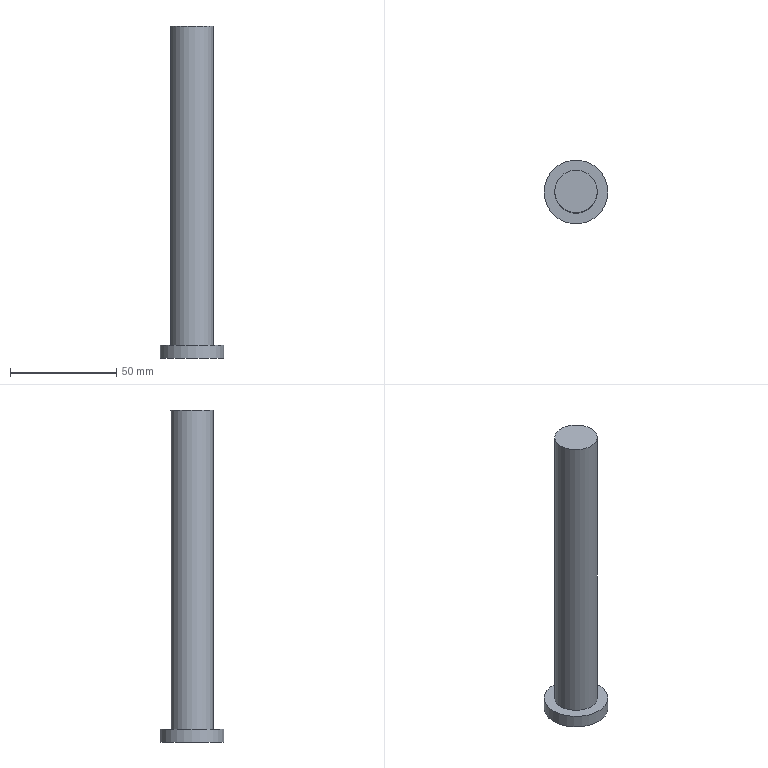Part | NX | features 侧推千斤顶活塞销 2 | 1 solid | 5 faces | box 30 x 30 x 156 mm | volume 51365 mm3 | plane 3 | cylinder 2 | commonest cylinder face diameters 20 x1 30 x1
STEP:
#1=CARTESIAN_POINT('',(10.,0.,150.));
#2=VERTEX_POINT('',#1);
#3=CARTESIAN_POINT('',(0.,0.,150.));
#4=DIRECTION('',(0.,0.,1.));
#5=DIRECTION('',(1.,0.,0.));
#6=AXIS2_PLACEMENT_3D('',#3,#4,#5);
#7=CIRCLE('',#6,10.);
#8=EDGE_CURVE('',#2,#2,#7,.T.);
#9=ORIENTED_EDGE('',*,*,#8,.F.);
#10=EDGE_LOOP('',(#9));
#11=FACE_BOUND('',#10,.T.);
#12=CARTESIAN_POINT('',(-10.,0.,0.));
#13=VERTEX_POINT('',#12);
#14=CARTESIAN_POINT('',(0.,0.,0.));
#15=DIRECTION('',(0.,0.,-1.));
#16=DIRECTION('',(-1.,0.,0.));
#17=AXIS2_PLACEMENT_3D('',#14,#15,#16);
#18=CIRCLE('',#17,10.);
#19=EDGE_CURVE('',#13,#13,#18,.T.);
#20=ORIENTED_EDGE('',*,*,#19,.F.);
#21=EDGE_LOOP('',(#20));
#22=FACE_BOUND('',#21,.T.);
#23=CARTESIAN_POINT('',(0.,0.,150.));
#24=DIRECTION('',(0.,0.,-1.));
#25=DIRECTION('',(-1.,0.,0.));
#26=AXIS2_PLACEMENT_3D('',#23,#24,#25);
#27=CYLINDRICAL_SURFACE('',#26,10.);
#28=ADVANCED_FACE('',(#11,#22),#27,.T.);
#29=ORIENTED_EDGE('',*,*,#8,.T.);
#30=EDGE_LOOP('',(#29));
#31=FACE_BOUND('',#30,.T.);
#32=CARTESIAN_POINT('',(0.,0.,150.));
#33=DIRECTION('',(0.,0.,1.));
#34=DIRECTION('',(1.,0.,0.));
#35=AXIS2_PLACEMENT_3D('',#32,#33,#34);
#36=PLANE('',#35);
#37=ADVANCED_FACE('',(#31),#36,.T.);
#38=CARTESIAN_POINT('',(-15.,0.,0.));
#39=VERTEX_POINT('',#38);
#40=CARTESIAN_POINT('',(0.,0.,0.));
#41=DIRECTION('',(0.,0.,-1.));
#42=DIRECTION('',(-1.,0.,0.));
#43=AXIS2_PLACEMENT_3D('',#40,#41,#42);
#44=CIRCLE('',#43,15.);
#45=EDGE_CURVE('',#39,#39,#44,.T.);
#46=ORIENTED_EDGE('',*,*,#45,.F.);
#47=EDGE_LOOP('',(#46));
#48=FACE_BOUND('',#47,.T.);
#49=ORIENTED_EDGE('',*,*,#19,.T.);
#50=EDGE_LOOP('',(#49));
#51=FACE_BOUND('',#50,.T.);
#52=CARTESIAN_POINT('',(0.,0.,0.));
#53=DIRECTION('',(0.,0.,-1.));
#54=DIRECTION('',(-1.,0.,0.));
#55=AXIS2_PLACEMENT_3D('',#52,#53,#54);
#56=PLANE('',#55);
#57=ADVANCED_FACE('',(#48,#51),#56,.F.);
#58=CARTESIAN_POINT('',(-15.,0.,-6.));
#59=VERTEX_POINT('',#58);
#60=CARTESIAN_POINT('',(0.,0.,-6.));
#61=DIRECTION('',(0.,0.,-1.));
#62=DIRECTION('',(-1.,0.,0.));
#63=AXIS2_PLACEMENT_3D('',#60,#61,#62);
#64=CIRCLE('',#63,15.);
#65=EDGE_CURVE('',#59,#59,#64,.T.);
#66=ORIENTED_EDGE('',*,*,#65,.F.);
#67=EDGE_LOOP('',(#66));
#68=FACE_BOUND('',#67,.T.);
#69=ORIENTED_EDGE('',*,*,#45,.T.);
#70=EDGE_LOOP('',(#69));
#71=FACE_BOUND('',#70,.T.);
#72=CARTESIAN_POINT('',(0.,0.,-6.));
#73=DIRECTION('',(0.,0.,1.));
#74=DIRECTION('',(1.,0.,0.));
#75=AXIS2_PLACEMENT_3D('',#72,#73,#74);
#76=CYLINDRICAL_SURFACE('',#75,15.);
#77=ADVANCED_FACE('',(#68,#71),#76,.T.);
#78=ORIENTED_EDGE('',*,*,#65,.T.);
#79=EDGE_LOOP('',(#78));
#80=FACE_BOUND('',#79,.T.);
#81=CARTESIAN_POINT('',(0.,0.,-6.));
#82=DIRECTION('',(0.,0.,-1.));
#83=DIRECTION('',(-1.,0.,0.));
#84=AXIS2_PLACEMENT_3D('',#81,#82,#83);
#85=PLANE('',#84);
#86=ADVANCED_FACE('',(#80),#85,.T.);
#87=CLOSED_SHELL('',(#28,#37,#57,#77,#86));
#88=MANIFOLD_SOLID_BREP('',#87);
#89=(LENGTH_UNIT()NAMED_UNIT(*)SI_UNIT(.MILLI.,.METRE.));
#90=UNCERTAINTY_MEASURE_WITH_UNIT(LENGTH_MEASURE(0.00001),#89,'','');
#91=(NAMED_UNIT(*)PLANE_ANGLE_UNIT()SI_UNIT($,.RADIAN.));
#92=(NAMED_UNIT(*)SI_UNIT($,.STERADIAN.)SOLID_ANGLE_UNIT());
#93=(GEOMETRIC_REPRESENTATION_CONTEXT(3)GLOBAL_UNCERTAINTY_ASSIGNED_CONTEXT((#90))GLOBAL_UNIT_ASSIGNED_CONTEXT((#89,#91,#92))REPRESENTATION_CONTEXT('',''));
#94=ADVANCED_BREP_SHAPE_REPRESENTATION('',(#88),#93);